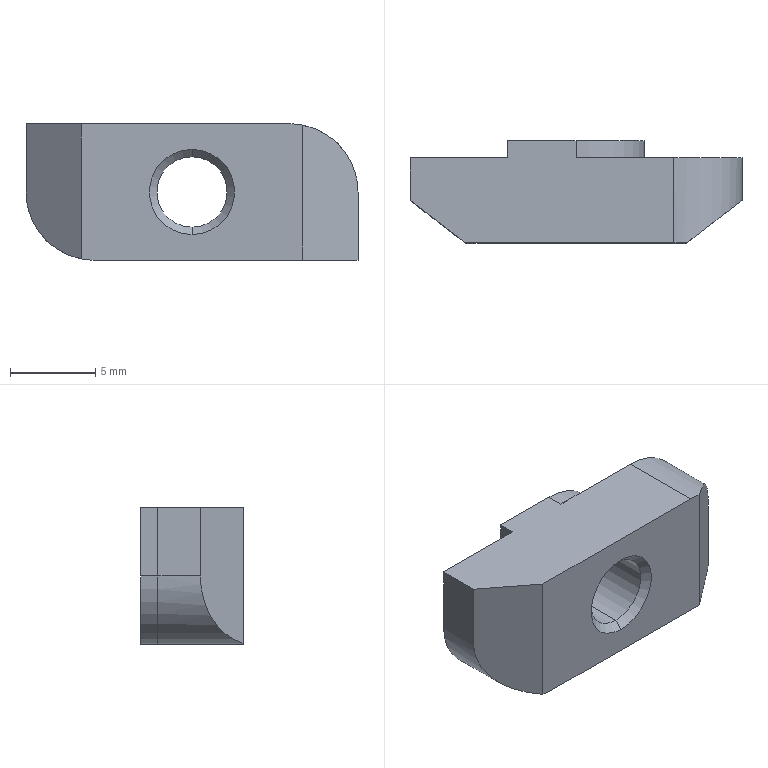Part | SolidWorks | features BaseBody 1 | 1 solid | 22 faces | box 19.5 x 6 x 8 mm | volume 667.11 mm3 | plane 12 | cylinder 6 | cone 4 | commonest cylinder face diameters 8 x4 4.134 x2
STEP:
#1=CARTESIAN_POINT('',(9.75,0.433,-1.933));
#2=VERTEX_POINT('',#1);
#3=CARTESIAN_POINT('',(9.75,0.433,-6.067));
#4=VERTEX_POINT('',#3);
#5=CARTESIAN_POINT('',(9.75,0.433,-4.));
#6=DIRECTION('',(0.,-1.,0.));
#7=DIRECTION('',(0.,0.,-1.));
#8=AXIS2_PLACEMENT_3D('',#5,#6,#7);
#9=CIRCLE('',#8,2.067);
#10=EDGE_CURVE('',#2,#4,#9,.T.);
#11=ORIENTED_EDGE('',*,*,#10,.F.);
#12=CARTESIAN_POINT('',(9.75,0.,-1.5));
#13=VERTEX_POINT('',#12);
#14=CARTESIAN_POINT('',(9.75,0.,-1.5));
#15=DIRECTION('',(0.,-0.7071,0.7071));
#16=VECTOR('',#15,1000.);
#17=LINE('',#14,#16);
#18=EDGE_CURVE('',#2,#13,#17,.T.);
#19=ORIENTED_EDGE('',*,*,#18,.T.);
#20=CARTESIAN_POINT('',(9.75,0.,-6.5));
#21=VERTEX_POINT('',#20);
#22=CARTESIAN_POINT('',(9.75,0.,-4.));
#23=DIRECTION('',(0.,-1.,0.));
#24=DIRECTION('',(0.,0.,-1.));
#25=AXIS2_PLACEMENT_3D('',#22,#23,#24);
#26=CIRCLE('',#25,2.5);
#27=EDGE_CURVE('',#13,#21,#26,.T.);
#28=ORIENTED_EDGE('',*,*,#27,.T.);
#29=CARTESIAN_POINT('',(9.75,0.,-6.5));
#30=DIRECTION('',(0.,-0.7071,-0.7071));
#31=VECTOR('',#30,1000.);
#32=LINE('',#29,#31);
#33=EDGE_CURVE('',#4,#21,#32,.T.);
#34=ORIENTED_EDGE('',*,*,#33,.F.);
#35=EDGE_LOOP('',(#11,#19,#28,#34));
#36=FACE_OUTER_BOUND('',#35,.T.);
#37=CARTESIAN_POINT('',(9.75,0.,-4.));
#38=DIRECTION('',(0.,-1.,0.));
#39=DIRECTION('',(0.,0.,-1.));
#40=AXIS2_PLACEMENT_3D('',#37,#38,#39);
#41=CONICAL_SURFACE('',#40,2.5,0.7854);
#42=ADVANCED_FACE('',(#36),#41,.F.);
#43=ORIENTED_EDGE('',*,*,#10,.T.);
#44=CARTESIAN_POINT('',(9.75,5.567,-6.067));
#45=VERTEX_POINT('',#44);
#46=CARTESIAN_POINT('',(9.75,0.,-6.067));
#47=DIRECTION('',(0.,1.,0.));
#48=VECTOR('',#47,1000.);
#49=LINE('',#46,#48);
#50=EDGE_CURVE('',#4,#45,#49,.T.);
#51=ORIENTED_EDGE('',*,*,#50,.T.);
#52=CARTESIAN_POINT('',(9.75,5.567,-1.933));
#53=VERTEX_POINT('',#52);
#54=CARTESIAN_POINT('',(9.75,5.567,-4.));
#55=DIRECTION('',(0.,-1.,0.));
#56=DIRECTION('',(0.,0.,1.));
#57=AXIS2_PLACEMENT_3D('',#54,#55,#56);
#58=CIRCLE('',#57,2.067);
#59=EDGE_CURVE('',#53,#45,#58,.T.);
#60=ORIENTED_EDGE('',*,*,#59,.F.);
#61=CARTESIAN_POINT('',(9.75,0.,-1.933));
#62=DIRECTION('',(0.,1.,0.));
#63=VECTOR('',#62,1000.);
#64=LINE('',#61,#63);
#65=EDGE_CURVE('',#2,#53,#64,.T.);
#66=ORIENTED_EDGE('',*,*,#65,.F.);
#67=EDGE_LOOP('',(#43,#51,#60,#66));
#68=FACE_OUTER_BOUND('',#67,.T.);
#69=CARTESIAN_POINT('',(9.75,0.,-4.));
#70=DIRECTION('',(0.,1.,0.));
#71=DIRECTION('',(0.,0.,1.));
#72=AXIS2_PLACEMENT_3D('',#69,#70,#71);
#73=CYLINDRICAL_SURFACE('',#72,2.067);
#74=ADVANCED_FACE('',(#68),#73,.F.);
#75=ORIENTED_EDGE('',*,*,#59,.T.);
#76=CARTESIAN_POINT('',(9.75,6.,-6.5));
#77=VERTEX_POINT('',#76);
#78=CARTESIAN_POINT('',(9.75,6.,-6.5));
#79=DIRECTION('',(0.,0.7071,-0.7071));
#80=VECTOR('',#79,1000.);
#81=LINE('',#78,#80);
#82=EDGE_CURVE('',#45,#77,#81,.T.);
#83=ORIENTED_EDGE('',*,*,#82,.T.);
#84=CARTESIAN_POINT('',(9.75,6.,-1.5));
#85=VERTEX_POINT('',#84);
#86=CARTESIAN_POINT('',(9.75,6.,-4.));
#87=DIRECTION('',(0.,-1.,0.));
#88=DIRECTION('',(0.,0.,1.));
#89=AXIS2_PLACEMENT_3D('',#86,#87,#88);
#90=CIRCLE('',#89,2.5);
#91=EDGE_CURVE('',#85,#77,#90,.T.);
#92=ORIENTED_EDGE('',*,*,#91,.F.);
#93=CARTESIAN_POINT('',(9.75,6.,-1.5));
#94=DIRECTION('',(0.,0.7071,0.7071));
#95=VECTOR('',#94,1000.);
#96=LINE('',#93,#95);
#97=EDGE_CURVE('',#53,#85,#96,.T.);
#98=ORIENTED_EDGE('',*,*,#97,.F.);
#99=EDGE_LOOP('',(#75,#83,#92,#98));
#100=FACE_OUTER_BOUND('',#99,.T.);
#101=CARTESIAN_POINT('',(9.75,6.,-4.));
#102=DIRECTION('',(0.,1.,0.));
#103=DIRECTION('',(0.,0.,1.));
#104=AXIS2_PLACEMENT_3D('',#101,#102,#103);
#105=CONICAL_SURFACE('',#104,2.5,0.7854);
#106=ADVANCED_FACE('',(#100),#105,.F.);
#107=CARTESIAN_POINT('',(9.75,0.,-4.));
#108=DIRECTION('',(0.,-1.,0.));
#109=DIRECTION('',(0.,0.,-1.));
#110=AXIS2_PLACEMENT_3D('',#107,#108,#109);
#111=CIRCLE('',#110,2.5);
#112=EDGE_CURVE('',#21,#13,#111,.T.);
#113=ORIENTED_EDGE('',*,*,#112,.F.);
#114=ORIENTED_EDGE('',*,*,#27,.F.);
#115=EDGE_LOOP('',(#113,#114));
#116=FACE_BOUND('',#115,.T.);
#117=CARTESIAN_POINT('',(16.25,0.,-0.07094));
#118=VERTEX_POINT('',#117);
#119=CARTESIAN_POINT('',(16.25,0.,-8.));
#120=VERTEX_POINT('',#119);
#121=CARTESIAN_POINT('',(16.25,0.,-4.));
#122=DIRECTION('',(0.,0.,-1.));
#123=VECTOR('',#122,1000.);
#124=LINE('',#121,#123);
#125=EDGE_CURVE('',#118,#120,#124,.T.);
#126=ORIENTED_EDGE('',*,*,#125,.F.);
#127=CARTESIAN_POINT('',(15.5,0.,0.));
#128=VERTEX_POINT('',#127);
#129=CARTESIAN_POINT('',(15.5,0.,-4.));
#130=DIRECTION('',(0.,1.,0.));
#131=DIRECTION('',(0.,0.,1.));
#132=AXIS2_PLACEMENT_3D('',#129,#130,#131);
#133=CIRCLE('',#132,4.);
#134=EDGE_CURVE('',#128,#118,#133,.T.);
#135=ORIENTED_EDGE('',*,*,#134,.F.);
#136=CARTESIAN_POINT('',(3.25,0.,0.));
#137=VERTEX_POINT('',#136);
#138=CARTESIAN_POINT('',(15.5,0.,0.));
#139=DIRECTION('',(1.,0.,0.));
#140=VECTOR('',#139,1000.);
#141=LINE('',#138,#140);
#142=EDGE_CURVE('',#137,#128,#141,.T.);
#143=ORIENTED_EDGE('',*,*,#142,.F.);
#144=CARTESIAN_POINT('',(3.25,0.,-7.929));
#145=VERTEX_POINT('',#144);
#146=CARTESIAN_POINT('',(3.25,0.,-4.));
#147=DIRECTION('',(0.,0.,1.));
#148=VECTOR('',#147,1000.);
#149=LINE('',#146,#148);
#150=EDGE_CURVE('',#145,#137,#149,.T.);
#151=ORIENTED_EDGE('',*,*,#150,.F.);
#152=CARTESIAN_POINT('',(4.,0.,-8.));
#153=VERTEX_POINT('',#152);
#154=CARTESIAN_POINT('',(4.,0.,-4.));
#155=DIRECTION('',(0.,1.,0.));
#156=DIRECTION('',(0.,0.,1.));
#157=AXIS2_PLACEMENT_3D('',#154,#155,#156);
#158=CIRCLE('',#157,4.);
#159=EDGE_CURVE('',#153,#145,#158,.T.);
#160=ORIENTED_EDGE('',*,*,#159,.F.);
#161=CARTESIAN_POINT('',(15.5,0.,-8.));
#162=DIRECTION('',(-1.,0.,0.));
#163=VECTOR('',#162,1000.);
#164=LINE('',#161,#163);
#165=EDGE_CURVE('',#120,#153,#164,.T.);
#166=ORIENTED_EDGE('',*,*,#165,.F.);
#167=EDGE_LOOP('',(#126,#135,#143,#151,#160,#166));
#168=FACE_OUTER_BOUND('',#167,.T.);
#169=CARTESIAN_POINT('',(15.5,0.,-4.));
#170=DIRECTION('',(0.,1.,0.));
#171=DIRECTION('',(0.,0.,1.));
#172=AXIS2_PLACEMENT_3D('',#169,#170,#171);
#173=PLANE('',#172);
#174=ADVANCED_FACE('',(#116,#168),#173,.F.);
#175=ORIENTED_EDGE('',*,*,#18,.F.);
#176=CARTESIAN_POINT('',(9.75,0.433,-4.));
#177=DIRECTION('',(0.,-1.,0.));
#178=DIRECTION('',(0.,0.,-1.));
#179=AXIS2_PLACEMENT_3D('',#176,#177,#178);
#180=CIRCLE('',#179,2.067);
#181=EDGE_CURVE('',#4,#2,#180,.T.);
#182=ORIENTED_EDGE('',*,*,#181,.F.);
#183=ORIENTED_EDGE('',*,*,#33,.T.);
#184=ORIENTED_EDGE('',*,*,#112,.T.);
#185=EDGE_LOOP('',(#175,#182,#183,#184));
#186=FACE_OUTER_BOUND('',#185,.T.);
#187=CARTESIAN_POINT('',(9.75,0.,-4.));
#188=DIRECTION('',(0.,-1.,0.));
#189=DIRECTION('',(0.,0.,-1.));
#190=AXIS2_PLACEMENT_3D('',#187,#188,#189);
#191=CONICAL_SURFACE('',#190,2.5,0.7854);
#192=ADVANCED_FACE('',(#186),#191,.F.);
#193=CARTESIAN_POINT('',(19.5,2.5,-8.));
#194=VERTEX_POINT('',#193);
#195=CARTESIAN_POINT('',(16.25,0.,-8.));
#196=DIRECTION('',(0.7926,0.6097,0.));
#197=VECTOR('',#196,1000.);
#198=LINE('',#195,#197);
#199=EDGE_CURVE('',#120,#194,#198,.T.);
#200=ORIENTED_EDGE('',*,*,#199,.F.);
#201=ORIENTED_EDGE('',*,*,#165,.T.);
#202=CARTESIAN_POINT('',(4.,5.,-8.));
#203=VERTEX_POINT('',#202);
#204=CARTESIAN_POINT('',(4.,5.,-8.));
#205=DIRECTION('',(0.,-1.,0.));
#206=VECTOR('',#205,1000.);
#207=LINE('',#204,#206);
#208=EDGE_CURVE('',#203,#153,#207,.T.);
#209=ORIENTED_EDGE('',*,*,#208,.F.);
#210=CARTESIAN_POINT('',(9.75,5.,-8.));
#211=VERTEX_POINT('',#210);
#212=CARTESIAN_POINT('',(19.5,5.,-8.));
#213=DIRECTION('',(-1.,0.,0.));
#214=VECTOR('',#213,1000.);
#215=LINE('',#212,#214);
#216=EDGE_CURVE('',#211,#203,#215,.T.);
#217=ORIENTED_EDGE('',*,*,#216,.F.);
#218=CARTESIAN_POINT('',(9.75,6.,-8.));
#219=VERTEX_POINT('',#218);
#220=CARTESIAN_POINT('',(9.75,6.,-8.));
#221=DIRECTION('',(0.,-1.,0.));
#222=VECTOR('',#221,1000.);
#223=LINE('',#220,#222);
#224=EDGE_CURVE('',#219,#211,#223,.T.);
#225=ORIENTED_EDGE('',*,*,#224,.F.);
#226=CARTESIAN_POINT('',(13.75,6.,-8.));
#227=VERTEX_POINT('',#226);
#228=CARTESIAN_POINT('',(19.5,6.,-8.));
#229=DIRECTION('',(-1.,0.,0.));
#230=VECTOR('',#229,1000.);
#231=LINE('',#228,#230);
#232=EDGE_CURVE('',#227,#219,#231,.T.);
#233=ORIENTED_EDGE('',*,*,#232,.F.);
#234=CARTESIAN_POINT('',(13.75,5.,-8.));
#235=VERTEX_POINT('',#234);
#236=CARTESIAN_POINT('',(13.75,6.,-8.));
#237=DIRECTION('',(0.,-1.,0.));
#238=VECTOR('',#237,1000.);
#239=LINE('',#236,#238);
#240=EDGE_CURVE('',#227,#235,#239,.T.);
#241=ORIENTED_EDGE('',*,*,#240,.T.);
#242=CARTESIAN_POINT('',(19.5,5.,-8.));
#243=VERTEX_POINT('',#242);
#244=CARTESIAN_POINT('',(19.5,5.,-8.));
#245=DIRECTION('',(-1.,0.,0.));
#246=VECTOR('',#245,1000.);
#247=LINE('',#244,#246);
#248=EDGE_CURVE('',#243,#235,#247,.T.);
#249=ORIENTED_EDGE('',*,*,#248,.F.);
#250=CARTESIAN_POINT('',(19.5,5.,-8.));
#251=DIRECTION('',(0.,1.,0.));
#252=VECTOR('',#251,1000.);
#253=LINE('',#250,#252);
#254=EDGE_CURVE('',#194,#243,#253,.T.);
#255=ORIENTED_EDGE('',*,*,#254,.F.);
#256=EDGE_LOOP('',(#200,#201,#209,#217,#225,#233,#241,#249,#255));
#257=FACE_OUTER_BOUND('',#256,.T.);
#258=CARTESIAN_POINT('',(19.5,5.,-8.));
#259=DIRECTION('',(0.,0.,1.));
#260=DIRECTION('',(1.,0.,0.));
#261=AXIS2_PLACEMENT_3D('',#258,#259,#260);
#262=PLANE('',#261);
#263=ADVANCED_FACE('',(#257),#262,.F.);
#264=ORIENTED_EDGE('',*,*,#199,.T.);
#265=CARTESIAN_POINT('',(19.5,2.5,-4.));
#266=VERTEX_POINT('',#265);
#267=CARTESIAN_POINT('',(19.5,2.5,-10.));
#268=DIRECTION('',(0.,0.,-1.));
#269=VECTOR('',#268,1000.);
#270=LINE('',#267,#269);
#271=EDGE_CURVE('',#266,#194,#270,.T.);
#272=ORIENTED_EDGE('',*,*,#271,.F.);
#273=CARTESIAN_POINT('',(16.25,0.,-0.07094));
#274=CARTESIAN_POINT('',(18.221,1.516,-0.4472));
#275=CARTESIAN_POINT('',(19.5,2.5,-1.993));
#276=CARTESIAN_POINT('',(19.5,2.5,-4.));
#277=(BOUNDED_CURVE()B_SPLINE_CURVE(3,(#273,#274,#275,#276),.UNSPECIFIED.,.F.,.F.)B_SPLINE_CURVE_WITH_KNOTS((4,4),(4.901,6.283),.UNSPECIFIED.)CURVE()GEOMETRIC_REPRESENTATION_ITEM()RATIONAL_B_SPLINE_CURVE((1.,0.847,0.847,1.))REPRESENTATION_ITEM(''));
#278=EDGE_CURVE('',#118,#266,#277,.T.);
#279=ORIENTED_EDGE('',*,*,#278,.F.);
#280=ORIENTED_EDGE('',*,*,#125,.T.);
#281=EDGE_LOOP('',(#264,#272,#279,#280));
#282=FACE_OUTER_BOUND('',#281,.T.);
#283=CARTESIAN_POINT('',(19.5,2.5,-10.));
#284=DIRECTION('',(-0.6097,0.7926,0.));
#285=DIRECTION('',(-0.7926,-0.6097,0.));
#286=AXIS2_PLACEMENT_3D('',#283,#284,#285);
#287=PLANE('',#286);
#288=ADVANCED_FACE('',(#282),#287,.F.);
#289=CARTESIAN_POINT('',(0.,2.5,0.));
#290=VERTEX_POINT('',#289);
#291=CARTESIAN_POINT('',(3.25,0.,0.));
#292=DIRECTION('',(-0.7926,0.6097,0.));
#293=VECTOR('',#292,1000.);
#294=LINE('',#291,#293);
#295=EDGE_CURVE('',#137,#290,#294,.T.);
#296=ORIENTED_EDGE('',*,*,#295,.F.);
#297=ORIENTED_EDGE('',*,*,#142,.T.);
#298=CARTESIAN_POINT('',(15.5,5.,0.));
#299=VERTEX_POINT('',#298);
#300=CARTESIAN_POINT('',(15.5,5.,0.));
#301=DIRECTION('',(0.,-1.,0.));
#302=VECTOR('',#301,1000.);
#303=LINE('',#300,#302);
#304=EDGE_CURVE('',#299,#128,#303,.T.);
#305=ORIENTED_EDGE('',*,*,#304,.F.);
#306=CARTESIAN_POINT('',(9.75,5.,0.));
#307=VERTEX_POINT('',#306);
#308=CARTESIAN_POINT('',(0.,5.,0.));
#309=DIRECTION('',(1.,0.,0.));
#310=VECTOR('',#309,1000.);
#311=LINE('',#308,#310);
#312=EDGE_CURVE('',#307,#299,#311,.T.);
#313=ORIENTED_EDGE('',*,*,#312,.F.);
#314=CARTESIAN_POINT('',(9.75,6.,0.));
#315=VERTEX_POINT('',#314);
#316=CARTESIAN_POINT('',(9.75,6.,0.));
#317=DIRECTION('',(0.,-1.,0.));
#318=VECTOR('',#317,1000.);
#319=LINE('',#316,#318);
#320=EDGE_CURVE('',#315,#307,#319,.T.);
#321=ORIENTED_EDGE('',*,*,#320,.F.);
#322=CARTESIAN_POINT('',(5.75,6.,0.));
#323=VERTEX_POINT('',#322);
#324=CARTESIAN_POINT('',(0.,6.,0.));
#325=DIRECTION('',(1.,0.,0.));
#326=VECTOR('',#325,1000.);
#327=LINE('',#324,#326);
#328=EDGE_CURVE('',#323,#315,#327,.T.);
#329=ORIENTED_EDGE('',*,*,#328,.F.);
#330=CARTESIAN_POINT('',(5.75,5.,0.));
#331=VERTEX_POINT('',#330);
#332=CARTESIAN_POINT('',(5.75,6.,0.));
#333=DIRECTION('',(0.,-1.,0.));
#334=VECTOR('',#333,1000.);
#335=LINE('',#332,#334);
#336=EDGE_CURVE('',#323,#331,#335,.T.);
#337=ORIENTED_EDGE('',*,*,#336,.T.);
#338=CARTESIAN_POINT('',(0.,5.,0.));
#339=VERTEX_POINT('',#338);
#340=CARTESIAN_POINT('',(0.,5.,0.));
#341=DIRECTION('',(1.,0.,0.));
#342=VECTOR('',#341,1000.);
#343=LINE('',#340,#342);
#344=EDGE_CURVE('',#339,#331,#343,.T.);
#345=ORIENTED_EDGE('',*,*,#344,.F.);
#346=CARTESIAN_POINT('',(0.,5.,0.));
#347=DIRECTION('',(0.,1.,0.));
#348=VECTOR('',#347,1000.);
#349=LINE('',#346,#348);
#350=EDGE_CURVE('',#290,#339,#349,.T.);
#351=ORIENTED_EDGE('',*,*,#350,.F.);
#352=EDGE_LOOP('',(#296,#297,#305,#313,#321,#329,#337,#345,#351));
#353=FACE_OUTER_BOUND('',#352,.T.);
#354=CARTESIAN_POINT('',(0.,5.,0.));
#355=DIRECTION('',(0.,0.,-1.));
#356=DIRECTION('',(-1.,0.,0.));
#357=AXIS2_PLACEMENT_3D('',#354,#355,#356);
#358=PLANE('',#357);
#359=ADVANCED_FACE('',(#353),#358,.F.);
#360=ORIENTED_EDGE('',*,*,#295,.T.);
#361=CARTESIAN_POINT('',(0.,2.5,-4.));
#362=VERTEX_POINT('',#361);
#363=CARTESIAN_POINT('',(0.,2.5,-10.));
#364=DIRECTION('',(0.,0.,1.));
#365=VECTOR('',#364,1000.);
#366=LINE('',#363,#365);
#367=EDGE_CURVE('',#362,#290,#366,.T.);
#368=ORIENTED_EDGE('',*,*,#367,.F.);
#369=CARTESIAN_POINT('',(3.25,0.,-7.929));
#370=CARTESIAN_POINT('',(1.279,1.516,-7.553));
#371=CARTESIAN_POINT('',(0.,2.5,-6.007));
#372=CARTESIAN_POINT('',(0.,2.5,-4.));
#373=(BOUNDED_CURVE()B_SPLINE_CURVE(3,(#369,#370,#371,#372),.UNSPECIFIED.,.F.,.T.)B_SPLINE_CURVE_WITH_KNOTS((4,4),(4.901,6.283),.UNSPECIFIED.)CURVE()GEOMETRIC_REPRESENTATION_ITEM()RATIONAL_B_SPLINE_CURVE((1.,0.847,0.847,1.))REPRESENTATION_ITEM(''));
#374=EDGE_CURVE('',#145,#362,#373,.T.);
#375=ORIENTED_EDGE('',*,*,#374,.F.);
#376=ORIENTED_EDGE('',*,*,#150,.T.);
#377=EDGE_LOOP('',(#360,#368,#375,#376));
#378=FACE_OUTER_BOUND('',#377,.T.);
#379=CARTESIAN_POINT('',(3.25,0.,-10.));
#380=DIRECTION('',(0.6097,0.7926,0.));
#381=DIRECTION('',(-0.7926,0.6097,0.));
#382=AXIS2_PLACEMENT_3D('',#379,#380,#381);
#383=PLANE('',#382);
#384=ADVANCED_FACE('',(#378),#383,.F.);
#385=ORIENTED_EDGE('',*,*,#50,.F.);
#386=ORIENTED_EDGE('',*,*,#181,.T.);
#387=ORIENTED_EDGE('',*,*,#65,.T.);
#388=CARTESIAN_POINT('',(9.75,5.567,-4.));
#389=DIRECTION('',(0.,-1.,0.));
#390=DIRECTION('',(0.,0.,1.));
#391=AXIS2_PLACEMENT_3D('',#388,#389,#390);
#392=CIRCLE('',#391,2.067);
#393=EDGE_CURVE('',#45,#53,#392,.T.);
#394=ORIENTED_EDGE('',*,*,#393,.F.);
#395=EDGE_LOOP('',(#385,#386,#387,#394));
#396=FACE_OUTER_BOUND('',#395,.T.);
#397=CARTESIAN_POINT('',(9.75,0.,-4.));
#398=DIRECTION('',(0.,1.,0.));
#399=DIRECTION('',(0.,0.,1.));
#400=AXIS2_PLACEMENT_3D('',#397,#398,#399);
#401=CYLINDRICAL_SURFACE('',#400,2.067);
#402=ADVANCED_FACE('',(#396),#401,.F.);
#403=ORIENTED_EDGE('',*,*,#271,.T.);
#404=ORIENTED_EDGE('',*,*,#254,.T.);
#405=CARTESIAN_POINT('',(19.5,5.,-4.));
#406=VERTEX_POINT('',#405);
#407=CARTESIAN_POINT('',(19.5,5.,-4.));
#408=DIRECTION('',(0.,0.,-1.));
#409=VECTOR('',#408,1000.);
#410=LINE('',#407,#409);
#411=EDGE_CURVE('',#406,#243,#410,.T.);
#412=ORIENTED_EDGE('',*,*,#411,.F.);
#413=CARTESIAN_POINT('',(19.5,5.,-4.));
#414=DIRECTION('',(0.,1.,0.));
#415=VECTOR('',#414,1000.);
#416=LINE('',#413,#415);
#417=EDGE_CURVE('',#266,#406,#416,.T.);
#418=ORIENTED_EDGE('',*,*,#417,.F.);
#419=EDGE_LOOP('',(#403,#404,#412,#418));
#420=FACE_OUTER_BOUND('',#419,.T.);
#421=CARTESIAN_POINT('',(19.5,5.,-4.));
#422=DIRECTION('',(-1.,0.,0.));
#423=DIRECTION('',(0.,0.,1.));
#424=AXIS2_PLACEMENT_3D('',#421,#422,#423);
#425=PLANE('',#424);
#426=ADVANCED_FACE('',(#420),#425,.F.);
#427=CARTESIAN_POINT('',(0.,5.,-4.));
#428=VERTEX_POINT('',#427);
#429=CARTESIAN_POINT('',(4.,5.,-4.));
#430=DIRECTION('',(0.,-1.,0.));
#431=DIRECTION('',(0.,0.,1.));
#432=AXIS2_PLACEMENT_3D('',#429,#430,#431);
#433=CIRCLE('',#432,4.);
#434=EDGE_CURVE('',#428,#203,#433,.T.);
#435=ORIENTED_EDGE('',*,*,#434,.T.);
#436=ORIENTED_EDGE('',*,*,#208,.T.);
#437=ORIENTED_EDGE('',*,*,#159,.T.);
#438=ORIENTED_EDGE('',*,*,#374,.T.);
#439=CARTESIAN_POINT('',(0.,5.,-4.));
#440=DIRECTION('',(0.,1.,0.));
#441=VECTOR('',#440,1000.);
#442=LINE('',#439,#441);
#443=EDGE_CURVE('',#362,#428,#442,.T.);
#444=ORIENTED_EDGE('',*,*,#443,.T.);
#445=EDGE_LOOP('',(#435,#436,#437,#438,#444));
#446=FACE_OUTER_BOUND('',#445,.T.);
#447=CARTESIAN_POINT('',(4.,5.,-4.));
#448=DIRECTION('',(0.,1.,0.));
#449=DIRECTION('',(0.,0.,1.));
#450=AXIS2_PLACEMENT_3D('',#447,#448,#449);
#451=CYLINDRICAL_SURFACE('',#450,4.);
#452=ADVANCED_FACE('',(#446),#451,.T.);
#453=CARTESIAN_POINT('',(0.,5.,-4.));
#454=DIRECTION('',(0.,0.,1.));
#455=VECTOR('',#454,1000.);
#456=LINE('',#453,#455);
#457=EDGE_CURVE('',#428,#339,#456,.T.);
#458=ORIENTED_EDGE('',*,*,#457,.T.);
#459=ORIENTED_EDGE('',*,*,#344,.T.);
#460=CARTESIAN_POINT('',(5.75,5.,-4.));
#461=VERTEX_POINT('',#460);
#462=CARTESIAN_POINT('',(5.75,5.,-4.));
#463=DIRECTION('',(0.,0.,-1.));
#464=VECTOR('',#463,1000.);
#465=LINE('',#462,#464);
#466=EDGE_CURVE('',#331,#461,#465,.T.);
#467=ORIENTED_EDGE('',*,*,#466,.T.);
#468=CARTESIAN_POINT('',(9.75,5.,-4.));
#469=DIRECTION('',(0.,-1.,0.));
#470=DIRECTION('',(0.,0.,1.));
#471=AXIS2_PLACEMENT_3D('',#468,#469,#470);
#472=CIRCLE('',#471,4.);
#473=EDGE_CURVE('',#461,#211,#472,.T.);
#474=ORIENTED_EDGE('',*,*,#473,.T.);
#475=ORIENTED_EDGE('',*,*,#216,.T.);
#476=ORIENTED_EDGE('',*,*,#434,.F.);
#477=EDGE_LOOP('',(#458,#459,#467,#474,#475,#476));
#478=FACE_OUTER_BOUND('',#477,.T.);
#479=CARTESIAN_POINT('',(15.5,5.,-4.));
#480=DIRECTION('',(0.,1.,0.));
#481=DIRECTION('',(0.,0.,1.));
#482=AXIS2_PLACEMENT_3D('',#479,#480,#481);
#483=PLANE('',#482);
#484=ADVANCED_FACE('',(#478),#483,.T.);
#485=ORIENTED_EDGE('',*,*,#91,.T.);
#486=CARTESIAN_POINT('',(9.75,6.,-4.));
#487=DIRECTION('',(0.,-1.,0.));
#488=DIRECTION('',(0.,0.,1.));
#489=AXIS2_PLACEMENT_3D('',#486,#487,#488);
#490=CIRCLE('',#489,2.5);
#491=EDGE_CURVE('',#77,#85,#490,.T.);
#492=ORIENTED_EDGE('',*,*,#491,.T.);
#493=EDGE_LOOP('',(#485,#492));
#494=FACE_BOUND('',#493,.T.);
#495=ORIENTED_EDGE('',*,*,#232,.T.);
#496=CARTESIAN_POINT('',(5.75,6.,-4.));
#497=VERTEX_POINT('',#496);
#498=CARTESIAN_POINT('',(9.75,6.,-4.));
#499=DIRECTION('',(0.,1.,0.));
#500=DIRECTION('',(0.,0.,1.));
#501=AXIS2_PLACEMENT_3D('',#498,#499,#500);
#502=CIRCLE('',#501,4.);
#503=EDGE_CURVE('',#219,#497,#502,.T.);
#504=ORIENTED_EDGE('',*,*,#503,.T.);
#505=CARTESIAN_POINT('',(5.75,6.,-4.));
#506=DIRECTION('',(0.,0.,1.));
#507=VECTOR('',#506,1000.);
#508=LINE('',#505,#507);
#509=EDGE_CURVE('',#497,#323,#508,.T.);
#510=ORIENTED_EDGE('',*,*,#509,.T.);
#511=ORIENTED_EDGE('',*,*,#328,.T.);
#512=CARTESIAN_POINT('',(13.75,6.,-4.));
#513=VERTEX_POINT('',#512);
#514=CARTESIAN_POINT('',(9.75,6.,-4.));
#515=DIRECTION('',(0.,1.,0.));
#516=DIRECTION('',(0.,0.,1.));
#517=AXIS2_PLACEMENT_3D('',#514,#515,#516);
#518=CIRCLE('',#517,4.);
#519=EDGE_CURVE('',#315,#513,#518,.T.);
#520=ORIENTED_EDGE('',*,*,#519,.T.);
#521=CARTESIAN_POINT('',(13.75,6.,-4.));
#522=DIRECTION('',(0.,0.,-1.));
#523=VECTOR('',#522,1000.);
#524=LINE('',#521,#523);
#525=EDGE_CURVE('',#513,#227,#524,.T.);
#526=ORIENTED_EDGE('',*,*,#525,.T.);
#527=EDGE_LOOP('',(#495,#504,#510,#511,#520,#526));
#528=FACE_OUTER_BOUND('',#527,.T.);
#529=CARTESIAN_POINT('',(9.75,6.,-4.));
#530=DIRECTION('',(0.,1.,0.));
#531=DIRECTION('',(0.,0.,1.));
#532=AXIS2_PLACEMENT_3D('',#529,#530,#531);
#533=PLANE('',#532);
#534=ADVANCED_FACE('',(#494,#528),#533,.T.);
#535=ORIENTED_EDGE('',*,*,#411,.T.);
#536=ORIENTED_EDGE('',*,*,#248,.T.);
#537=CARTESIAN_POINT('',(13.75,5.,-4.));
#538=VERTEX_POINT('',#537);
#539=CARTESIAN_POINT('',(13.75,5.,-4.));
#540=DIRECTION('',(0.,0.,1.));
#541=VECTOR('',#540,1000.);
#542=LINE('',#539,#541);
#543=EDGE_CURVE('',#235,#538,#542,.T.);
#544=ORIENTED_EDGE('',*,*,#543,.T.);
#545=CARTESIAN_POINT('',(9.75,5.,-4.));
#546=DIRECTION('',(0.,-1.,0.));
#547=DIRECTION('',(0.,0.,1.));
#548=AXIS2_PLACEMENT_3D('',#545,#546,#547);
#549=CIRCLE('',#548,4.);
#550=EDGE_CURVE('',#538,#307,#549,.T.);
#551=ORIENTED_EDGE('',*,*,#550,.T.);
#552=ORIENTED_EDGE('',*,*,#312,.T.);
#553=CARTESIAN_POINT('',(15.5,5.,-4.));
#554=DIRECTION('',(0.,1.,0.));
#555=DIRECTION('',(0.,0.,1.));
#556=AXIS2_PLACEMENT_3D('',#553,#554,#555);
#557=CIRCLE('',#556,4.);
#558=EDGE_CURVE('',#299,#406,#557,.T.);
#559=ORIENTED_EDGE('',*,*,#558,.T.);
#560=EDGE_LOOP('',(#535,#536,#544,#551,#552,#559));
#561=FACE_OUTER_BOUND('',#560,.T.);
#562=CARTESIAN_POINT('',(15.5,5.,-4.));
#563=DIRECTION('',(0.,1.,0.));
#564=DIRECTION('',(0.,0.,1.));
#565=AXIS2_PLACEMENT_3D('',#562,#563,#564);
#566=PLANE('',#565);
#567=ADVANCED_FACE('',(#561),#566,.T.);
#568=ORIENTED_EDGE('',*,*,#558,.F.);
#569=ORIENTED_EDGE('',*,*,#304,.T.);
#570=ORIENTED_EDGE('',*,*,#134,.T.);
#571=ORIENTED_EDGE('',*,*,#278,.T.);
#572=ORIENTED_EDGE('',*,*,#417,.T.);
#573=EDGE_LOOP('',(#568,#569,#570,#571,#572));
#574=FACE_OUTER_BOUND('',#573,.T.);
#575=CARTESIAN_POINT('',(15.5,5.,-4.));
#576=DIRECTION('',(0.,1.,0.));
#577=DIRECTION('',(0.,0.,1.));
#578=AXIS2_PLACEMENT_3D('',#575,#576,#577);
#579=CYLINDRICAL_SURFACE('',#578,4.);
#580=ADVANCED_FACE('',(#574),#579,.T.);
#581=ORIENTED_EDGE('',*,*,#367,.T.);
#582=ORIENTED_EDGE('',*,*,#350,.T.);
#583=ORIENTED_EDGE('',*,*,#457,.F.);
#584=ORIENTED_EDGE('',*,*,#443,.F.);
#585=EDGE_LOOP('',(#581,#582,#583,#584));
#586=FACE_OUTER_BOUND('',#585,.T.);
#587=CARTESIAN_POINT('',(0.,5.,-4.));
#588=DIRECTION('',(1.,0.,0.));
#589=DIRECTION('',(0.,0.,-1.));
#590=AXIS2_PLACEMENT_3D('',#587,#588,#589);
#591=PLANE('',#590);
#592=ADVANCED_FACE('',(#586),#591,.F.);
#593=ORIENTED_EDGE('',*,*,#82,.F.);
#594=ORIENTED_EDGE('',*,*,#393,.T.);
#595=ORIENTED_EDGE('',*,*,#97,.T.);
#596=ORIENTED_EDGE('',*,*,#491,.F.);
#597=EDGE_LOOP('',(#593,#594,#595,#596));
#598=FACE_OUTER_BOUND('',#597,.T.);
#599=CARTESIAN_POINT('',(9.75,6.,-4.));
#600=DIRECTION('',(0.,1.,0.));
#601=DIRECTION('',(0.,0.,1.));
#602=AXIS2_PLACEMENT_3D('',#599,#600,#601);
#603=CONICAL_SURFACE('',#602,2.5,0.7854);
#604=ADVANCED_FACE('',(#598),#603,.F.);
#605=ORIENTED_EDGE('',*,*,#503,.F.);
#606=ORIENTED_EDGE('',*,*,#224,.T.);
#607=ORIENTED_EDGE('',*,*,#473,.F.);
#608=CARTESIAN_POINT('',(5.75,6.,-4.));
#609=DIRECTION('',(0.,1.,0.));
#610=VECTOR('',#609,1000.);
#611=LINE('',#608,#610);
#612=EDGE_CURVE('',#461,#497,#611,.T.);
#613=ORIENTED_EDGE('',*,*,#612,.T.);
#614=EDGE_LOOP('',(#605,#606,#607,#613));
#615=FACE_OUTER_BOUND('',#614,.T.);
#616=CARTESIAN_POINT('',(9.75,6.,-4.));
#617=DIRECTION('',(0.,1.,0.));
#618=DIRECTION('',(0.,0.,1.));
#619=AXIS2_PLACEMENT_3D('',#616,#617,#618);
#620=CYLINDRICAL_SURFACE('',#619,4.);
#621=ADVANCED_FACE('',(#615),#620,.T.);
#622=ORIENTED_EDGE('',*,*,#336,.F.);
#623=ORIENTED_EDGE('',*,*,#509,.F.);
#624=ORIENTED_EDGE('',*,*,#612,.F.);
#625=ORIENTED_EDGE('',*,*,#466,.F.);
#626=EDGE_LOOP('',(#622,#623,#624,#625));
#627=FACE_OUTER_BOUND('',#626,.T.);
#628=CARTESIAN_POINT('',(5.75,6.,-4.));
#629=DIRECTION('',(1.,0.,0.));
#630=DIRECTION('',(0.,0.,-1.));
#631=AXIS2_PLACEMENT_3D('',#628,#629,#630);
#632=PLANE('',#631);
#633=ADVANCED_FACE('',(#627),#632,.F.);
#634=ORIENTED_EDGE('',*,*,#240,.F.);
#635=ORIENTED_EDGE('',*,*,#525,.F.);
#636=CARTESIAN_POINT('',(13.75,6.,-4.));
#637=DIRECTION('',(0.,1.,0.));
#638=VECTOR('',#637,1000.);
#639=LINE('',#636,#638);
#640=EDGE_CURVE('',#538,#513,#639,.T.);
#641=ORIENTED_EDGE('',*,*,#640,.F.);
#642=ORIENTED_EDGE('',*,*,#543,.F.);
#643=EDGE_LOOP('',(#634,#635,#641,#642));
#644=FACE_OUTER_BOUND('',#643,.T.);
#645=CARTESIAN_POINT('',(13.75,6.,-4.));
#646=DIRECTION('',(-1.,0.,0.));
#647=DIRECTION('',(0.,0.,1.));
#648=AXIS2_PLACEMENT_3D('',#645,#646,#647);
#649=PLANE('',#648);
#650=ADVANCED_FACE('',(#644),#649,.F.);
#651=ORIENTED_EDGE('',*,*,#519,.F.);
#652=ORIENTED_EDGE('',*,*,#320,.T.);
#653=ORIENTED_EDGE('',*,*,#550,.F.);
#654=ORIENTED_EDGE('',*,*,#640,.T.);
#655=EDGE_LOOP('',(#651,#652,#653,#654));
#656=FACE_OUTER_BOUND('',#655,.T.);
#657=CARTESIAN_POINT('',(9.75,6.,-4.));
#658=DIRECTION('',(0.,1.,0.));
#659=DIRECTION('',(0.,0.,1.));
#660=AXIS2_PLACEMENT_3D('',#657,#658,#659);
#661=CYLINDRICAL_SURFACE('',#660,4.);
#662=ADVANCED_FACE('',(#656),#661,.T.);
#663=CLOSED_SHELL('',(#42,#74,#106,#174,#192,#263,#288,#359,#384,#402,#426,#452,#484,#534,#567,#580,#592,#604,#621,#633,#650,#662));
#664=MANIFOLD_SOLID_BREP('',#663);
#665=CARTESIAN_POINT('',(0.,0.,0.));
#666=DIRECTION('',(0.,0.,1.));
#667=DIRECTION('',(1.,0.,0.));
#668=AXIS2_PLACEMENT_3D('',#665,#666,#667);
#669=(LENGTH_UNIT()NAMED_UNIT(*)SI_UNIT(.MILLI.,.METRE.));
#670=UNCERTAINTY_MEASURE_WITH_UNIT(LENGTH_MEASURE(0.00001),#669,'','');
#671=(NAMED_UNIT(*)PLANE_ANGLE_UNIT()SI_UNIT($,.RADIAN.));
#672=(NAMED_UNIT(*)SI_UNIT($,.STERADIAN.)SOLID_ANGLE_UNIT());
#673=(GEOMETRIC_REPRESENTATION_CONTEXT(3)GLOBAL_UNCERTAINTY_ASSIGNED_CONTEXT((#670))GLOBAL_UNIT_ASSIGNED_CONTEXT((#669,#671,#672))REPRESENTATION_CONTEXT('',''));
#674=ADVANCED_BREP_SHAPE_REPRESENTATION('',(#664,#668),#673);